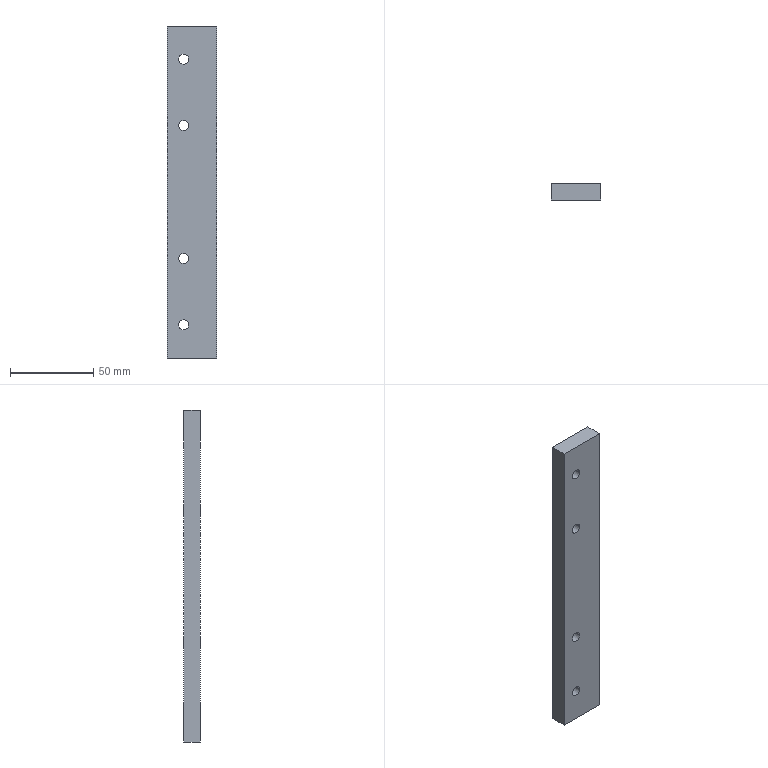Part | SolidWorks | features BaseBody 1 | 1 solid | 14 faces | box 30 x 10 x 200 mm | volume 58869 mm3 | cylinder 8 | plane 6 | commonest cylinder face diameters 6 x8
STEP:
#1=CARTESIAN_POINT('',(260.959,37.138,40.));
#2=VERTEX_POINT('',#1);
#3=CARTESIAN_POINT('',(266.959,37.138,40.));
#4=VERTEX_POINT('',#3);
#5=CARTESIAN_POINT('',(263.959,37.138,40.));
#6=DIRECTION('',(0.,-1.,0.));
#7=DIRECTION('',(0.,0.,1.));
#8=AXIS2_PLACEMENT_3D('',#5,#6,#7);
#9=CIRCLE('',#8,3.);
#10=EDGE_CURVE('',#2,#4,#9,.T.);
#11=ORIENTED_EDGE('',*,*,#10,.T.);
#12=CARTESIAN_POINT('',(266.959,47.138,40.));
#13=VERTEX_POINT('',#12);
#14=CARTESIAN_POINT('',(266.959,27.138,40.));
#15=DIRECTION('',(0.,1.,0.));
#16=VECTOR('',#15,1000.);
#17=LINE('',#14,#16);
#18=EDGE_CURVE('',#4,#13,#17,.T.);
#19=ORIENTED_EDGE('',*,*,#18,.T.);
#20=CARTESIAN_POINT('',(260.959,47.138,40.));
#21=VERTEX_POINT('',#20);
#22=CARTESIAN_POINT('',(263.959,47.138,40.));
#23=DIRECTION('',(0.,1.,0.));
#24=DIRECTION('',(1.,0.,0.));
#25=AXIS2_PLACEMENT_3D('',#22,#23,#24);
#26=CIRCLE('',#25,3.);
#27=EDGE_CURVE('',#13,#21,#26,.T.);
#28=ORIENTED_EDGE('',*,*,#27,.T.);
#29=CARTESIAN_POINT('',(260.959,27.138,40.));
#30=DIRECTION('',(0.,1.,0.));
#31=VECTOR('',#30,1000.);
#32=LINE('',#29,#31);
#33=EDGE_CURVE('',#2,#21,#32,.T.);
#34=ORIENTED_EDGE('',*,*,#33,.F.);
#35=EDGE_LOOP('',(#11,#19,#28,#34));
#36=FACE_OUTER_BOUND('',#35,.T.);
#37=CARTESIAN_POINT('',(263.959,27.138,40.));
#38=DIRECTION('',(0.,1.,0.));
#39=DIRECTION('',(-1.,0.,0.));
#40=AXIS2_PLACEMENT_3D('',#37,#38,#39);
#41=CYLINDRICAL_SURFACE('',#40,3.);
#42=ADVANCED_FACE('',(#36),#41,.F.);
#43=CARTESIAN_POINT('',(260.959,37.138,80.));
#44=VERTEX_POINT('',#43);
#45=CARTESIAN_POINT('',(266.959,37.138,80.));
#46=VERTEX_POINT('',#45);
#47=CARTESIAN_POINT('',(263.959,37.138,80.));
#48=DIRECTION('',(0.,-1.,0.));
#49=DIRECTION('',(0.,0.,1.));
#50=AXIS2_PLACEMENT_3D('',#47,#48,#49);
#51=CIRCLE('',#50,3.);
#52=EDGE_CURVE('',#44,#46,#51,.T.);
#53=ORIENTED_EDGE('',*,*,#52,.T.);
#54=CARTESIAN_POINT('',(266.959,47.138,80.));
#55=VERTEX_POINT('',#54);
#56=CARTESIAN_POINT('',(266.959,27.138,80.));
#57=DIRECTION('',(0.,1.,0.));
#58=VECTOR('',#57,1000.);
#59=LINE('',#56,#58);
#60=EDGE_CURVE('',#46,#55,#59,.T.);
#61=ORIENTED_EDGE('',*,*,#60,.T.);
#62=CARTESIAN_POINT('',(260.959,47.138,80.));
#63=VERTEX_POINT('',#62);
#64=CARTESIAN_POINT('',(263.959,47.138,80.));
#65=DIRECTION('',(0.,1.,0.));
#66=DIRECTION('',(1.,0.,0.));
#67=AXIS2_PLACEMENT_3D('',#64,#65,#66);
#68=CIRCLE('',#67,3.);
#69=EDGE_CURVE('',#55,#63,#68,.T.);
#70=ORIENTED_EDGE('',*,*,#69,.T.);
#71=CARTESIAN_POINT('',(260.959,27.138,80.));
#72=DIRECTION('',(0.,1.,0.));
#73=VECTOR('',#72,1000.);
#74=LINE('',#71,#73);
#75=EDGE_CURVE('',#44,#63,#74,.T.);
#76=ORIENTED_EDGE('',*,*,#75,.F.);
#77=EDGE_LOOP('',(#53,#61,#70,#76));
#78=FACE_OUTER_BOUND('',#77,.T.);
#79=CARTESIAN_POINT('',(263.959,27.138,80.));
#80=DIRECTION('',(0.,1.,0.));
#81=DIRECTION('',(-1.,0.,0.));
#82=AXIS2_PLACEMENT_3D('',#79,#80,#81);
#83=CYLINDRICAL_SURFACE('',#82,3.);
#84=ADVANCED_FACE('',(#78),#83,.F.);
#85=CARTESIAN_POINT('',(260.959,37.138,-80.));
#86=VERTEX_POINT('',#85);
#87=CARTESIAN_POINT('',(266.959,37.138,-80.));
#88=VERTEX_POINT('',#87);
#89=CARTESIAN_POINT('',(263.959,37.138,-80.));
#90=DIRECTION('',(0.,-1.,0.));
#91=DIRECTION('',(0.,0.,1.));
#92=AXIS2_PLACEMENT_3D('',#89,#90,#91);
#93=CIRCLE('',#92,3.);
#94=EDGE_CURVE('',#86,#88,#93,.T.);
#95=ORIENTED_EDGE('',*,*,#94,.T.);
#96=CARTESIAN_POINT('',(266.959,47.138,-80.));
#97=VERTEX_POINT('',#96);
#98=CARTESIAN_POINT('',(266.959,27.138,-80.));
#99=DIRECTION('',(0.,1.,0.));
#100=VECTOR('',#99,1000.);
#101=LINE('',#98,#100);
#102=EDGE_CURVE('',#88,#97,#101,.T.);
#103=ORIENTED_EDGE('',*,*,#102,.T.);
#104=CARTESIAN_POINT('',(260.959,47.138,-80.));
#105=VERTEX_POINT('',#104);
#106=CARTESIAN_POINT('',(263.959,47.138,-80.));
#107=DIRECTION('',(0.,1.,0.));
#108=DIRECTION('',(-1.,0.,0.));
#109=AXIS2_PLACEMENT_3D('',#106,#107,#108);
#110=CIRCLE('',#109,3.);
#111=EDGE_CURVE('',#97,#105,#110,.T.);
#112=ORIENTED_EDGE('',*,*,#111,.T.);
#113=CARTESIAN_POINT('',(260.959,27.138,-80.));
#114=DIRECTION('',(0.,1.,0.));
#115=VECTOR('',#114,1000.);
#116=LINE('',#113,#115);
#117=EDGE_CURVE('',#86,#105,#116,.T.);
#118=ORIENTED_EDGE('',*,*,#117,.F.);
#119=EDGE_LOOP('',(#95,#103,#112,#118));
#120=FACE_OUTER_BOUND('',#119,.T.);
#121=CARTESIAN_POINT('',(263.959,27.138,-80.));
#122=DIRECTION('',(0.,1.,0.));
#123=DIRECTION('',(-1.,0.,0.));
#124=AXIS2_PLACEMENT_3D('',#121,#122,#123);
#125=CYLINDRICAL_SURFACE('',#124,3.);
#126=ADVANCED_FACE('',(#120),#125,.F.);
#127=CARTESIAN_POINT('',(260.959,37.138,-40.));
#128=VERTEX_POINT('',#127);
#129=CARTESIAN_POINT('',(266.959,37.138,-40.));
#130=VERTEX_POINT('',#129);
#131=CARTESIAN_POINT('',(263.959,37.138,-40.));
#132=DIRECTION('',(0.,-1.,0.));
#133=DIRECTION('',(0.,0.,1.));
#134=AXIS2_PLACEMENT_3D('',#131,#132,#133);
#135=CIRCLE('',#134,3.);
#136=EDGE_CURVE('',#128,#130,#135,.T.);
#137=ORIENTED_EDGE('',*,*,#136,.T.);
#138=CARTESIAN_POINT('',(266.959,47.138,-40.));
#139=VERTEX_POINT('',#138);
#140=CARTESIAN_POINT('',(266.959,27.138,-40.));
#141=DIRECTION('',(0.,1.,0.));
#142=VECTOR('',#141,1000.);
#143=LINE('',#140,#142);
#144=EDGE_CURVE('',#130,#139,#143,.T.);
#145=ORIENTED_EDGE('',*,*,#144,.T.);
#146=CARTESIAN_POINT('',(260.959,47.138,-40.));
#147=VERTEX_POINT('',#146);
#148=CARTESIAN_POINT('',(263.959,47.138,-40.));
#149=DIRECTION('',(0.,1.,0.));
#150=DIRECTION('',(-1.,0.,0.));
#151=AXIS2_PLACEMENT_3D('',#148,#149,#150);
#152=CIRCLE('',#151,3.);
#153=EDGE_CURVE('',#139,#147,#152,.T.);
#154=ORIENTED_EDGE('',*,*,#153,.T.);
#155=CARTESIAN_POINT('',(260.959,27.138,-40.));
#156=DIRECTION('',(0.,1.,0.));
#157=VECTOR('',#156,1000.);
#158=LINE('',#155,#157);
#159=EDGE_CURVE('',#128,#147,#158,.T.);
#160=ORIENTED_EDGE('',*,*,#159,.F.);
#161=EDGE_LOOP('',(#137,#145,#154,#160));
#162=FACE_OUTER_BOUND('',#161,.T.);
#163=CARTESIAN_POINT('',(263.959,27.138,-40.));
#164=DIRECTION('',(0.,1.,0.));
#165=DIRECTION('',(-1.,0.,0.));
#166=AXIS2_PLACEMENT_3D('',#163,#164,#165);
#167=CYLINDRICAL_SURFACE('',#166,3.);
#168=ADVANCED_FACE('',(#162),#167,.F.);
#169=CARTESIAN_POINT('',(283.959,37.138,-100.));
#170=VERTEX_POINT('',#169);
#171=CARTESIAN_POINT('',(253.959,37.138,-100.));
#172=VERTEX_POINT('',#171);
#173=CARTESIAN_POINT('',(283.959,37.138,-100.));
#174=DIRECTION('',(-1.,0.,0.));
#175=VECTOR('',#174,1000.);
#176=LINE('',#173,#175);
#177=EDGE_CURVE('',#170,#172,#176,.T.);
#178=ORIENTED_EDGE('',*,*,#177,.T.);
#179=CARTESIAN_POINT('',(253.959,47.138,-100.));
#180=VERTEX_POINT('',#179);
#181=CARTESIAN_POINT('',(253.959,37.138,-100.));
#182=DIRECTION('',(0.,1.,0.));
#183=VECTOR('',#182,1000.);
#184=LINE('',#181,#183);
#185=EDGE_CURVE('',#172,#180,#184,.T.);
#186=ORIENTED_EDGE('',*,*,#185,.T.);
#187=CARTESIAN_POINT('',(283.959,47.138,-100.));
#188=VERTEX_POINT('',#187);
#189=CARTESIAN_POINT('',(283.959,47.138,-100.));
#190=DIRECTION('',(-1.,0.,0.));
#191=VECTOR('',#190,1000.);
#192=LINE('',#189,#191);
#193=EDGE_CURVE('',#188,#180,#192,.T.);
#194=ORIENTED_EDGE('',*,*,#193,.F.);
#195=CARTESIAN_POINT('',(283.959,37.138,-100.));
#196=DIRECTION('',(0.,-1.,0.));
#197=VECTOR('',#196,1000.);
#198=LINE('',#195,#197);
#199=EDGE_CURVE('',#188,#170,#198,.T.);
#200=ORIENTED_EDGE('',*,*,#199,.T.);
#201=EDGE_LOOP('',(#178,#186,#194,#200));
#202=FACE_OUTER_BOUND('',#201,.T.);
#203=CARTESIAN_POINT('',(283.959,37.138,-100.));
#204=DIRECTION('',(0.,0.,-1.));
#205=DIRECTION('',(-1.,0.,0.));
#206=AXIS2_PLACEMENT_3D('',#203,#204,#205);
#207=PLANE('',#206);
#208=ADVANCED_FACE('',(#202),#207,.T.);
#209=CARTESIAN_POINT('',(263.959,47.138,40.));
#210=DIRECTION('',(0.,1.,0.));
#211=DIRECTION('',(1.,0.,0.));
#212=AXIS2_PLACEMENT_3D('',#209,#210,#211);
#213=CIRCLE('',#212,3.);
#214=EDGE_CURVE('',#21,#13,#213,.T.);
#215=ORIENTED_EDGE('',*,*,#214,.F.);
#216=ORIENTED_EDGE('',*,*,#27,.F.);
#217=EDGE_LOOP('',(#215,#216));
#218=FACE_BOUND('',#217,.T.);
#219=CARTESIAN_POINT('',(263.959,47.138,80.));
#220=DIRECTION('',(0.,1.,0.));
#221=DIRECTION('',(1.,0.,0.));
#222=AXIS2_PLACEMENT_3D('',#219,#220,#221);
#223=CIRCLE('',#222,3.);
#224=EDGE_CURVE('',#63,#55,#223,.T.);
#225=ORIENTED_EDGE('',*,*,#224,.F.);
#226=ORIENTED_EDGE('',*,*,#69,.F.);
#227=EDGE_LOOP('',(#225,#226));
#228=FACE_BOUND('',#227,.T.);
#229=CARTESIAN_POINT('',(263.959,47.138,-80.));
#230=DIRECTION('',(0.,1.,0.));
#231=DIRECTION('',(-1.,0.,0.));
#232=AXIS2_PLACEMENT_3D('',#229,#230,#231);
#233=CIRCLE('',#232,3.);
#234=EDGE_CURVE('',#105,#97,#233,.T.);
#235=ORIENTED_EDGE('',*,*,#234,.F.);
#236=ORIENTED_EDGE('',*,*,#111,.F.);
#237=EDGE_LOOP('',(#235,#236));
#238=FACE_BOUND('',#237,.T.);
#239=CARTESIAN_POINT('',(263.959,47.138,-40.));
#240=DIRECTION('',(0.,1.,0.));
#241=DIRECTION('',(-1.,0.,0.));
#242=AXIS2_PLACEMENT_3D('',#239,#240,#241);
#243=CIRCLE('',#242,3.);
#244=EDGE_CURVE('',#147,#139,#243,.T.);
#245=ORIENTED_EDGE('',*,*,#244,.F.);
#246=ORIENTED_EDGE('',*,*,#153,.F.);
#247=EDGE_LOOP('',(#245,#246));
#248=FACE_BOUND('',#247,.T.);
#249=ORIENTED_EDGE('',*,*,#193,.T.);
#250=CARTESIAN_POINT('',(253.959,47.138,100.));
#251=VERTEX_POINT('',#250);
#252=CARTESIAN_POINT('',(253.959,47.138,100.));
#253=DIRECTION('',(0.,0.,-1.));
#254=VECTOR('',#253,1000.);
#255=LINE('',#252,#254);
#256=EDGE_CURVE('',#251,#180,#255,.T.);
#257=ORIENTED_EDGE('',*,*,#256,.F.);
#258=CARTESIAN_POINT('',(283.959,47.138,100.));
#259=VERTEX_POINT('',#258);
#260=CARTESIAN_POINT('',(283.959,47.138,100.));
#261=DIRECTION('',(-1.,0.,0.));
#262=VECTOR('',#261,1000.);
#263=LINE('',#260,#262);
#264=EDGE_CURVE('',#259,#251,#263,.T.);
#265=ORIENTED_EDGE('',*,*,#264,.F.);
#266=CARTESIAN_POINT('',(283.959,47.138,-100.));
#267=DIRECTION('',(0.,0.,-1.));
#268=VECTOR('',#267,1000.);
#269=LINE('',#266,#268);
#270=EDGE_CURVE('',#259,#188,#269,.T.);
#271=ORIENTED_EDGE('',*,*,#270,.T.);
#272=EDGE_LOOP('',(#249,#257,#265,#271));
#273=FACE_OUTER_BOUND('',#272,.T.);
#274=CARTESIAN_POINT('',(283.959,47.138,-100.));
#275=DIRECTION('',(0.,1.,0.));
#276=DIRECTION('',(-1.,0.,0.));
#277=AXIS2_PLACEMENT_3D('',#274,#275,#276);
#278=PLANE('',#277);
#279=ADVANCED_FACE('',(#218,#228,#238,#248,#273),#278,.T.);
#280=ORIENTED_EDGE('',*,*,#264,.T.);
#281=CARTESIAN_POINT('',(253.959,37.138,100.));
#282=VERTEX_POINT('',#281);
#283=CARTESIAN_POINT('',(253.959,47.138,100.));
#284=DIRECTION('',(0.,-1.,0.));
#285=VECTOR('',#284,1000.);
#286=LINE('',#283,#285);
#287=EDGE_CURVE('',#251,#282,#286,.T.);
#288=ORIENTED_EDGE('',*,*,#287,.T.);
#289=CARTESIAN_POINT('',(283.959,37.138,100.));
#290=VERTEX_POINT('',#289);
#291=CARTESIAN_POINT('',(283.959,37.138,100.));
#292=DIRECTION('',(-1.,0.,0.));
#293=VECTOR('',#292,1000.);
#294=LINE('',#291,#293);
#295=EDGE_CURVE('',#290,#282,#294,.T.);
#296=ORIENTED_EDGE('',*,*,#295,.F.);
#297=CARTESIAN_POINT('',(283.959,47.138,100.));
#298=DIRECTION('',(0.,1.,0.));
#299=VECTOR('',#298,1000.);
#300=LINE('',#297,#299);
#301=EDGE_CURVE('',#290,#259,#300,.T.);
#302=ORIENTED_EDGE('',*,*,#301,.T.);
#303=EDGE_LOOP('',(#280,#288,#296,#302));
#304=FACE_OUTER_BOUND('',#303,.T.);
#305=CARTESIAN_POINT('',(283.959,47.138,100.));
#306=DIRECTION('',(0.,0.,1.));
#307=DIRECTION('',(0.,1.,0.));
#308=AXIS2_PLACEMENT_3D('',#305,#306,#307);
#309=PLANE('',#308);
#310=ADVANCED_FACE('',(#304),#309,.T.);
#311=ORIENTED_EDGE('',*,*,#10,.F.);
#312=CARTESIAN_POINT('',(263.959,37.138,40.));
#313=DIRECTION('',(0.,-1.,0.));
#314=DIRECTION('',(0.,0.,1.));
#315=AXIS2_PLACEMENT_3D('',#312,#313,#314);
#316=CIRCLE('',#315,3.);
#317=EDGE_CURVE('',#4,#2,#316,.T.);
#318=ORIENTED_EDGE('',*,*,#317,.F.);
#319=EDGE_LOOP('',(#311,#318));
#320=FACE_BOUND('',#319,.T.);
#321=ORIENTED_EDGE('',*,*,#52,.F.);
#322=CARTESIAN_POINT('',(263.959,37.138,80.));
#323=DIRECTION('',(0.,-1.,0.));
#324=DIRECTION('',(0.,0.,1.));
#325=AXIS2_PLACEMENT_3D('',#322,#323,#324);
#326=CIRCLE('',#325,3.);
#327=EDGE_CURVE('',#46,#44,#326,.T.);
#328=ORIENTED_EDGE('',*,*,#327,.F.);
#329=EDGE_LOOP('',(#321,#328));
#330=FACE_BOUND('',#329,.T.);
#331=ORIENTED_EDGE('',*,*,#94,.F.);
#332=CARTESIAN_POINT('',(263.959,37.138,-80.));
#333=DIRECTION('',(0.,-1.,0.));
#334=DIRECTION('',(0.,0.,1.));
#335=AXIS2_PLACEMENT_3D('',#332,#333,#334);
#336=CIRCLE('',#335,3.);
#337=EDGE_CURVE('',#88,#86,#336,.T.);
#338=ORIENTED_EDGE('',*,*,#337,.F.);
#339=EDGE_LOOP('',(#331,#338));
#340=FACE_BOUND('',#339,.T.);
#341=ORIENTED_EDGE('',*,*,#136,.F.);
#342=CARTESIAN_POINT('',(263.959,37.138,-40.));
#343=DIRECTION('',(0.,-1.,0.));
#344=DIRECTION('',(0.,0.,1.));
#345=AXIS2_PLACEMENT_3D('',#342,#343,#344);
#346=CIRCLE('',#345,3.);
#347=EDGE_CURVE('',#130,#128,#346,.T.);
#348=ORIENTED_EDGE('',*,*,#347,.F.);
#349=EDGE_LOOP('',(#341,#348));
#350=FACE_BOUND('',#349,.T.);
#351=ORIENTED_EDGE('',*,*,#295,.T.);
#352=CARTESIAN_POINT('',(253.959,37.138,100.));
#353=DIRECTION('',(0.,0.,-1.));
#354=VECTOR('',#353,1000.);
#355=LINE('',#352,#354);
#356=EDGE_CURVE('',#282,#172,#355,.T.);
#357=ORIENTED_EDGE('',*,*,#356,.T.);
#358=ORIENTED_EDGE('',*,*,#177,.F.);
#359=CARTESIAN_POINT('',(283.959,37.138,100.));
#360=DIRECTION('',(0.,0.,1.));
#361=VECTOR('',#360,1000.);
#362=LINE('',#359,#361);
#363=EDGE_CURVE('',#170,#290,#362,.T.);
#364=ORIENTED_EDGE('',*,*,#363,.T.);
#365=EDGE_LOOP('',(#351,#357,#358,#364));
#366=FACE_OUTER_BOUND('',#365,.T.);
#367=CARTESIAN_POINT('',(283.959,37.138,100.));
#368=DIRECTION('',(0.,-1.,0.));
#369=DIRECTION('',(0.,0.,1.));
#370=AXIS2_PLACEMENT_3D('',#367,#368,#369);
#371=PLANE('',#370);
#372=ADVANCED_FACE('',(#320,#330,#340,#350,#366),#371,.T.);
#373=ORIENTED_EDGE('',*,*,#199,.F.);
#374=ORIENTED_EDGE('',*,*,#270,.F.);
#375=ORIENTED_EDGE('',*,*,#301,.F.);
#376=ORIENTED_EDGE('',*,*,#363,.F.);
#377=EDGE_LOOP('',(#373,#374,#375,#376));
#378=FACE_OUTER_BOUND('',#377,.T.);
#379=CARTESIAN_POINT('',(283.959,173.862,121.393));
#380=DIRECTION('',(1.,0.,0.));
#381=DIRECTION('',(0.,0.,-1.));
#382=AXIS2_PLACEMENT_3D('',#379,#380,#381);
#383=PLANE('',#382);
#384=ADVANCED_FACE('',(#378),#383,.T.);
#385=ORIENTED_EDGE('',*,*,#256,.T.);
#386=ORIENTED_EDGE('',*,*,#185,.F.);
#387=ORIENTED_EDGE('',*,*,#356,.F.);
#388=ORIENTED_EDGE('',*,*,#287,.F.);
#389=EDGE_LOOP('',(#385,#386,#387,#388));
#390=FACE_OUTER_BOUND('',#389,.T.);
#391=CARTESIAN_POINT('',(253.959,173.862,121.393));
#392=DIRECTION('',(1.,0.,0.));
#393=DIRECTION('',(0.,0.,-1.));
#394=AXIS2_PLACEMENT_3D('',#391,#392,#393);
#395=PLANE('',#394);
#396=ADVANCED_FACE('',(#390),#395,.F.);
#397=ORIENTED_EDGE('',*,*,#144,.F.);
#398=ORIENTED_EDGE('',*,*,#347,.T.);
#399=ORIENTED_EDGE('',*,*,#159,.T.);
#400=ORIENTED_EDGE('',*,*,#244,.T.);
#401=EDGE_LOOP('',(#397,#398,#399,#400));
#402=FACE_OUTER_BOUND('',#401,.T.);
#403=CARTESIAN_POINT('',(263.959,27.138,-40.));
#404=DIRECTION('',(0.,1.,0.));
#405=DIRECTION('',(-1.,0.,0.));
#406=AXIS2_PLACEMENT_3D('',#403,#404,#405);
#407=CYLINDRICAL_SURFACE('',#406,3.);
#408=ADVANCED_FACE('',(#402),#407,.F.);
#409=ORIENTED_EDGE('',*,*,#102,.F.);
#410=ORIENTED_EDGE('',*,*,#337,.T.);
#411=ORIENTED_EDGE('',*,*,#117,.T.);
#412=ORIENTED_EDGE('',*,*,#234,.T.);
#413=EDGE_LOOP('',(#409,#410,#411,#412));
#414=FACE_OUTER_BOUND('',#413,.T.);
#415=CARTESIAN_POINT('',(263.959,27.138,-80.));
#416=DIRECTION('',(0.,1.,0.));
#417=DIRECTION('',(-1.,0.,0.));
#418=AXIS2_PLACEMENT_3D('',#415,#416,#417);
#419=CYLINDRICAL_SURFACE('',#418,3.);
#420=ADVANCED_FACE('',(#414),#419,.F.);
#421=ORIENTED_EDGE('',*,*,#60,.F.);
#422=ORIENTED_EDGE('',*,*,#327,.T.);
#423=ORIENTED_EDGE('',*,*,#75,.T.);
#424=ORIENTED_EDGE('',*,*,#224,.T.);
#425=EDGE_LOOP('',(#421,#422,#423,#424));
#426=FACE_OUTER_BOUND('',#425,.T.);
#427=CARTESIAN_POINT('',(263.959,27.138,80.));
#428=DIRECTION('',(0.,1.,0.));
#429=DIRECTION('',(-1.,0.,0.));
#430=AXIS2_PLACEMENT_3D('',#427,#428,#429);
#431=CYLINDRICAL_SURFACE('',#430,3.);
#432=ADVANCED_FACE('',(#426),#431,.F.);
#433=ORIENTED_EDGE('',*,*,#18,.F.);
#434=ORIENTED_EDGE('',*,*,#317,.T.);
#435=ORIENTED_EDGE('',*,*,#33,.T.);
#436=ORIENTED_EDGE('',*,*,#214,.T.);
#437=EDGE_LOOP('',(#433,#434,#435,#436));
#438=FACE_OUTER_BOUND('',#437,.T.);
#439=CARTESIAN_POINT('',(263.959,27.138,40.));
#440=DIRECTION('',(0.,1.,0.));
#441=DIRECTION('',(-1.,0.,0.));
#442=AXIS2_PLACEMENT_3D('',#439,#440,#441);
#443=CYLINDRICAL_SURFACE('',#442,3.);
#444=ADVANCED_FACE('',(#438),#443,.F.);
#445=CLOSED_SHELL('',(#42,#84,#126,#168,#208,#279,#310,#372,#384,#396,#408,#420,#432,#444));
#446=MANIFOLD_SOLID_BREP('',#445);
#447=CARTESIAN_POINT('',(0.,0.,0.));
#448=DIRECTION('',(0.,0.,1.));
#449=DIRECTION('',(1.,0.,0.));
#450=AXIS2_PLACEMENT_3D('',#447,#448,#449);
#451=(LENGTH_UNIT()NAMED_UNIT(*)SI_UNIT(.MILLI.,.METRE.));
#452=UNCERTAINTY_MEASURE_WITH_UNIT(LENGTH_MEASURE(0.00001),#451,'','');
#453=(NAMED_UNIT(*)PLANE_ANGLE_UNIT()SI_UNIT($,.RADIAN.));
#454=(NAMED_UNIT(*)SI_UNIT($,.STERADIAN.)SOLID_ANGLE_UNIT());
#455=(GEOMETRIC_REPRESENTATION_CONTEXT(3)GLOBAL_UNCERTAINTY_ASSIGNED_CONTEXT((#452))GLOBAL_UNIT_ASSIGNED_CONTEXT((#451,#453,#454))REPRESENTATION_CONTEXT('',''));
#456=ADVANCED_BREP_SHAPE_REPRESENTATION('',(#446,#450),#455);